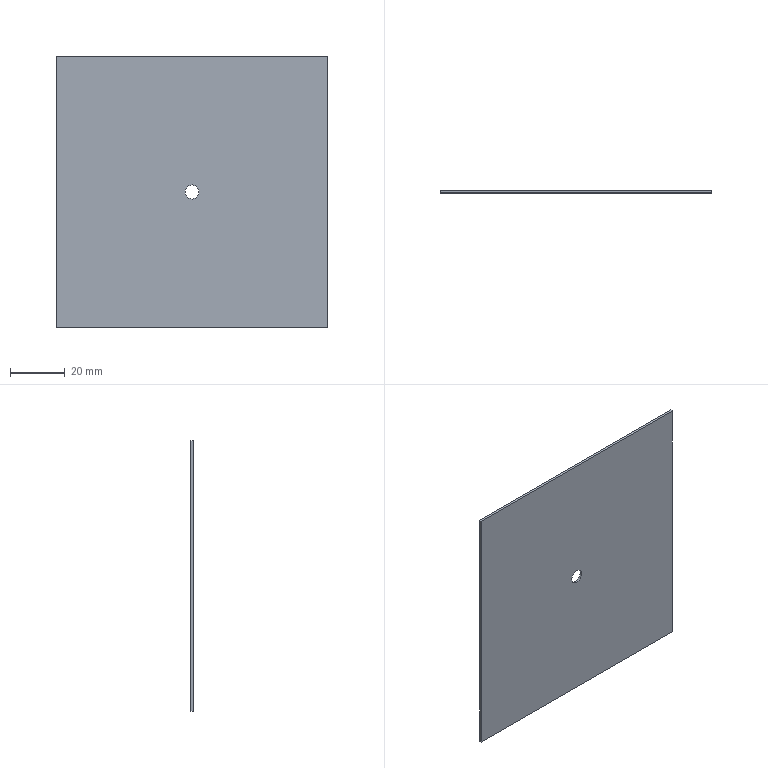Part | SolidWorks | features Extrusion 1 | 1 solid | 8 faces | box 98.4 x 0.8 x 98.4 mm | volume 7730 mm3 | plane 6 | cylinder 2 | commonest cylinder face diameters 5.1 x2
STEP:
#1=CARTESIAN_POINT('',(0.,0.8,-2.55));
#2=VERTEX_POINT('',#1);
#3=CARTESIAN_POINT('',(0.,0.8,2.55));
#4=VERTEX_POINT('',#3);
#5=CARTESIAN_POINT('',(0.,0.8,0.));
#6=DIRECTION('',(0.,1.,0.));
#7=DIRECTION('',(0.,0.,1.));
#8=AXIS2_PLACEMENT_3D('',#5,#6,#7);
#9=CIRCLE('',#8,2.55);
#10=EDGE_CURVE('',#2,#4,#9,.T.);
#11=ORIENTED_EDGE('',*,*,#10,.T.);
#12=CARTESIAN_POINT('',(0.,0.,2.55));
#13=VERTEX_POINT('',#12);
#14=CARTESIAN_POINT('',(0.,0.8,2.55));
#15=DIRECTION('',(0.,-1.,0.));
#16=VECTOR('',#15,1000.);
#17=LINE('',#14,#16);
#18=EDGE_CURVE('',#4,#13,#17,.T.);
#19=ORIENTED_EDGE('',*,*,#18,.T.);
#20=CARTESIAN_POINT('',(0.,0.,-2.55));
#21=VERTEX_POINT('',#20);
#22=CARTESIAN_POINT('',(0.,0.,0.));
#23=DIRECTION('',(0.,1.,0.));
#24=DIRECTION('',(0.,0.,1.));
#25=AXIS2_PLACEMENT_3D('',#22,#23,#24);
#26=CIRCLE('',#25,2.55);
#27=EDGE_CURVE('',#21,#13,#26,.T.);
#28=ORIENTED_EDGE('',*,*,#27,.F.);
#29=CARTESIAN_POINT('',(0.,0.8,-2.55));
#30=DIRECTION('',(0.,-1.,0.));
#31=VECTOR('',#30,1000.);
#32=LINE('',#29,#31);
#33=EDGE_CURVE('',#2,#21,#32,.T.);
#34=ORIENTED_EDGE('',*,*,#33,.F.);
#35=EDGE_LOOP('',(#11,#19,#28,#34));
#36=FACE_OUTER_BOUND('',#35,.T.);
#37=CARTESIAN_POINT('',(0.,0.8,0.));
#38=DIRECTION('',(0.,-1.,0.));
#39=DIRECTION('',(0.,0.,-1.));
#40=AXIS2_PLACEMENT_3D('',#37,#38,#39);
#41=CYLINDRICAL_SURFACE('',#40,2.55);
#42=ADVANCED_FACE('',(#36),#41,.F.);
#43=CARTESIAN_POINT('',(49.2,0.8,49.2));
#44=VERTEX_POINT('',#43);
#45=CARTESIAN_POINT('',(49.2,0.8,-49.2));
#46=VERTEX_POINT('',#45);
#47=CARTESIAN_POINT('',(49.2,0.8,49.2));
#48=DIRECTION('',(0.,0.,-1.));
#49=VECTOR('',#48,1000.);
#50=LINE('',#47,#49);
#51=EDGE_CURVE('',#44,#46,#50,.T.);
#52=ORIENTED_EDGE('',*,*,#51,.T.);
#53=CARTESIAN_POINT('',(-49.2,0.8,-49.2));
#54=VERTEX_POINT('',#53);
#55=CARTESIAN_POINT('',(-49.2,0.8,-49.2));
#56=DIRECTION('',(-1.,0.,0.));
#57=VECTOR('',#56,1000.);
#58=LINE('',#55,#57);
#59=EDGE_CURVE('',#46,#54,#58,.T.);
#60=ORIENTED_EDGE('',*,*,#59,.T.);
#61=CARTESIAN_POINT('',(-49.2,0.8,49.2));
#62=VERTEX_POINT('',#61);
#63=CARTESIAN_POINT('',(-49.2,0.8,49.2));
#64=DIRECTION('',(0.,0.,1.));
#65=VECTOR('',#64,1000.);
#66=LINE('',#63,#65);
#67=EDGE_CURVE('',#54,#62,#66,.T.);
#68=ORIENTED_EDGE('',*,*,#67,.T.);
#69=CARTESIAN_POINT('',(-49.2,0.8,49.2));
#70=DIRECTION('',(1.,0.,0.));
#71=VECTOR('',#70,1000.);
#72=LINE('',#69,#71);
#73=EDGE_CURVE('',#62,#44,#72,.T.);
#74=ORIENTED_EDGE('',*,*,#73,.T.);
#75=EDGE_LOOP('',(#52,#60,#68,#74));
#76=FACE_OUTER_BOUND('',#75,.T.);
#77=ORIENTED_EDGE('',*,*,#10,.F.);
#78=CARTESIAN_POINT('',(0.,0.8,0.));
#79=DIRECTION('',(0.,1.,0.));
#80=DIRECTION('',(0.,0.,1.));
#81=AXIS2_PLACEMENT_3D('',#78,#79,#80);
#82=CIRCLE('',#81,2.55);
#83=EDGE_CURVE('',#4,#2,#82,.T.);
#84=ORIENTED_EDGE('',*,*,#83,.F.);
#85=EDGE_LOOP('',(#77,#84));
#86=FACE_BOUND('',#85,.T.);
#87=CARTESIAN_POINT('',(0.,0.8,0.));
#88=DIRECTION('',(0.,-1.,0.));
#89=DIRECTION('',(0.,0.,-1.));
#90=AXIS2_PLACEMENT_3D('',#87,#88,#89);
#91=PLANE('',#90);
#92=ADVANCED_FACE('',(#76,#86),#91,.F.);
#93=CARTESIAN_POINT('',(49.2,0.,49.2));
#94=VERTEX_POINT('',#93);
#95=CARTESIAN_POINT('',(49.2,0.,-49.2));
#96=VERTEX_POINT('',#95);
#97=CARTESIAN_POINT('',(49.2,0.,49.2));
#98=DIRECTION('',(0.,0.,-1.));
#99=VECTOR('',#98,1000.);
#100=LINE('',#97,#99);
#101=EDGE_CURVE('',#94,#96,#100,.T.);
#102=ORIENTED_EDGE('',*,*,#101,.F.);
#103=CARTESIAN_POINT('',(-49.2,0.,49.2));
#104=VERTEX_POINT('',#103);
#105=CARTESIAN_POINT('',(-49.2,0.,49.2));
#106=DIRECTION('',(1.,0.,0.));
#107=VECTOR('',#106,1000.);
#108=LINE('',#105,#107);
#109=EDGE_CURVE('',#104,#94,#108,.T.);
#110=ORIENTED_EDGE('',*,*,#109,.F.);
#111=CARTESIAN_POINT('',(-49.2,0.,-49.2));
#112=VERTEX_POINT('',#111);
#113=CARTESIAN_POINT('',(-49.2,0.,49.2));
#114=DIRECTION('',(0.,0.,1.));
#115=VECTOR('',#114,1000.);
#116=LINE('',#113,#115);
#117=EDGE_CURVE('',#112,#104,#116,.T.);
#118=ORIENTED_EDGE('',*,*,#117,.F.);
#119=CARTESIAN_POINT('',(-49.2,0.,-49.2));
#120=DIRECTION('',(-1.,0.,0.));
#121=VECTOR('',#120,1000.);
#122=LINE('',#119,#121);
#123=EDGE_CURVE('',#96,#112,#122,.T.);
#124=ORIENTED_EDGE('',*,*,#123,.F.);
#125=EDGE_LOOP('',(#102,#110,#118,#124));
#126=FACE_OUTER_BOUND('',#125,.T.);
#127=ORIENTED_EDGE('',*,*,#27,.T.);
#128=CARTESIAN_POINT('',(0.,0.,0.));
#129=DIRECTION('',(0.,1.,0.));
#130=DIRECTION('',(0.,0.,1.));
#131=AXIS2_PLACEMENT_3D('',#128,#129,#130);
#132=CIRCLE('',#131,2.55);
#133=EDGE_CURVE('',#13,#21,#132,.T.);
#134=ORIENTED_EDGE('',*,*,#133,.T.);
#135=EDGE_LOOP('',(#127,#134));
#136=FACE_BOUND('',#135,.T.);
#137=CARTESIAN_POINT('',(0.,0.,0.));
#138=DIRECTION('',(0.,-1.,0.));
#139=DIRECTION('',(0.,0.,-1.));
#140=AXIS2_PLACEMENT_3D('',#137,#138,#139);
#141=PLANE('',#140);
#142=ADVANCED_FACE('',(#126,#136),#141,.T.);
#143=ORIENTED_EDGE('',*,*,#101,.T.);
#144=CARTESIAN_POINT('',(49.2,0.8,-49.2));
#145=DIRECTION('',(0.,-1.,0.));
#146=VECTOR('',#145,1000.);
#147=LINE('',#144,#146);
#148=EDGE_CURVE('',#46,#96,#147,.T.);
#149=ORIENTED_EDGE('',*,*,#148,.F.);
#150=ORIENTED_EDGE('',*,*,#51,.F.);
#151=CARTESIAN_POINT('',(49.2,0.8,49.2));
#152=DIRECTION('',(0.,-1.,0.));
#153=VECTOR('',#152,1000.);
#154=LINE('',#151,#153);
#155=EDGE_CURVE('',#44,#94,#154,.T.);
#156=ORIENTED_EDGE('',*,*,#155,.T.);
#157=EDGE_LOOP('',(#143,#149,#150,#156));
#158=FACE_OUTER_BOUND('',#157,.T.);
#159=CARTESIAN_POINT('',(49.2,0.8,49.2));
#160=DIRECTION('',(-1.,0.,0.));
#161=DIRECTION('',(0.,0.,1.));
#162=AXIS2_PLACEMENT_3D('',#159,#160,#161);
#163=PLANE('',#162);
#164=ADVANCED_FACE('',(#158),#163,.F.);
#165=ORIENTED_EDGE('',*,*,#123,.T.);
#166=CARTESIAN_POINT('',(-49.2,0.8,-49.2));
#167=DIRECTION('',(0.,-1.,0.));
#168=VECTOR('',#167,1000.);
#169=LINE('',#166,#168);
#170=EDGE_CURVE('',#54,#112,#169,.T.);
#171=ORIENTED_EDGE('',*,*,#170,.F.);
#172=ORIENTED_EDGE('',*,*,#59,.F.);
#173=ORIENTED_EDGE('',*,*,#148,.T.);
#174=EDGE_LOOP('',(#165,#171,#172,#173));
#175=FACE_OUTER_BOUND('',#174,.T.);
#176=CARTESIAN_POINT('',(-49.2,0.8,-49.2));
#177=DIRECTION('',(0.,0.,1.));
#178=DIRECTION('',(1.,0.,0.));
#179=AXIS2_PLACEMENT_3D('',#176,#177,#178);
#180=PLANE('',#179);
#181=ADVANCED_FACE('',(#175),#180,.F.);
#182=ORIENTED_EDGE('',*,*,#117,.T.);
#183=CARTESIAN_POINT('',(-49.2,0.8,49.2));
#184=DIRECTION('',(0.,-1.,0.));
#185=VECTOR('',#184,1000.);
#186=LINE('',#183,#185);
#187=EDGE_CURVE('',#62,#104,#186,.T.);
#188=ORIENTED_EDGE('',*,*,#187,.F.);
#189=ORIENTED_EDGE('',*,*,#67,.F.);
#190=ORIENTED_EDGE('',*,*,#170,.T.);
#191=EDGE_LOOP('',(#182,#188,#189,#190));
#192=FACE_OUTER_BOUND('',#191,.T.);
#193=CARTESIAN_POINT('',(-49.2,0.8,49.2));
#194=DIRECTION('',(1.,0.,0.));
#195=DIRECTION('',(0.,0.,-1.));
#196=AXIS2_PLACEMENT_3D('',#193,#194,#195);
#197=PLANE('',#196);
#198=ADVANCED_FACE('',(#192),#197,.F.);
#199=ORIENTED_EDGE('',*,*,#109,.T.);
#200=ORIENTED_EDGE('',*,*,#155,.F.);
#201=ORIENTED_EDGE('',*,*,#73,.F.);
#202=ORIENTED_EDGE('',*,*,#187,.T.);
#203=EDGE_LOOP('',(#199,#200,#201,#202));
#204=FACE_OUTER_BOUND('',#203,.T.);
#205=CARTESIAN_POINT('',(-49.2,0.8,49.2));
#206=DIRECTION('',(0.,0.,-1.));
#207=DIRECTION('',(-1.,0.,0.));
#208=AXIS2_PLACEMENT_3D('',#205,#206,#207);
#209=PLANE('',#208);
#210=ADVANCED_FACE('',(#204),#209,.F.);
#211=ORIENTED_EDGE('',*,*,#18,.F.);
#212=ORIENTED_EDGE('',*,*,#83,.T.);
#213=ORIENTED_EDGE('',*,*,#33,.T.);
#214=ORIENTED_EDGE('',*,*,#133,.F.);
#215=EDGE_LOOP('',(#211,#212,#213,#214));
#216=FACE_OUTER_BOUND('',#215,.T.);
#217=CARTESIAN_POINT('',(0.,0.8,0.));
#218=DIRECTION('',(0.,-1.,0.));
#219=DIRECTION('',(0.,0.,-1.));
#220=AXIS2_PLACEMENT_3D('',#217,#218,#219);
#221=CYLINDRICAL_SURFACE('',#220,2.55);
#222=ADVANCED_FACE('',(#216),#221,.F.);
#223=CLOSED_SHELL('',(#42,#92,#142,#164,#181,#198,#210,#222));
#224=MANIFOLD_SOLID_BREP('',#223);
#225=CARTESIAN_POINT('',(0.,0.,0.));
#226=DIRECTION('',(0.,0.,1.));
#227=DIRECTION('',(1.,0.,0.));
#228=AXIS2_PLACEMENT_3D('',#225,#226,#227);
#229=(LENGTH_UNIT()NAMED_UNIT(*)SI_UNIT(.MILLI.,.METRE.));
#230=UNCERTAINTY_MEASURE_WITH_UNIT(LENGTH_MEASURE(0.00001),#229,'','');
#231=(NAMED_UNIT(*)PLANE_ANGLE_UNIT()SI_UNIT($,.RADIAN.));
#232=(NAMED_UNIT(*)SI_UNIT($,.STERADIAN.)SOLID_ANGLE_UNIT());
#233=(GEOMETRIC_REPRESENTATION_CONTEXT(3)GLOBAL_UNCERTAINTY_ASSIGNED_CONTEXT((#230))GLOBAL_UNIT_ASSIGNED_CONTEXT((#229,#231,#232))REPRESENTATION_CONTEXT('',''));
#234=ADVANCED_BREP_SHAPE_REPRESENTATION('',(#224,#228),#233);